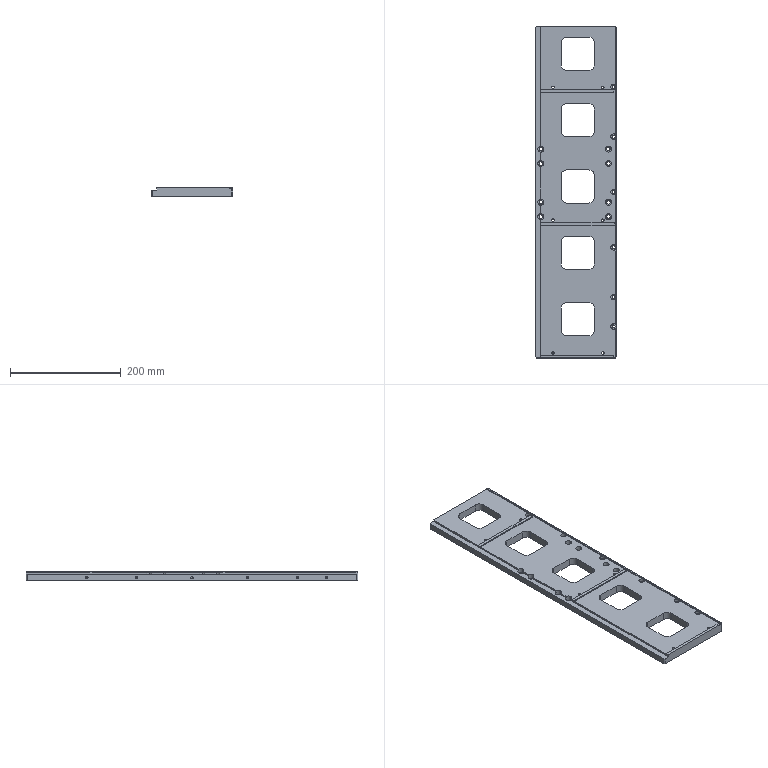Part | STEP file | XL-01 | 1 solid | 200 faces | box 148 x 600 x 16 mm | volume 970586 mm3 | cylinder 112 | plane 76 | cone 12 | commonest cylinder face diameters 20 x20 6.6 x16 10.8 x16 4.2 x12 4.5 x12 5.5 x12